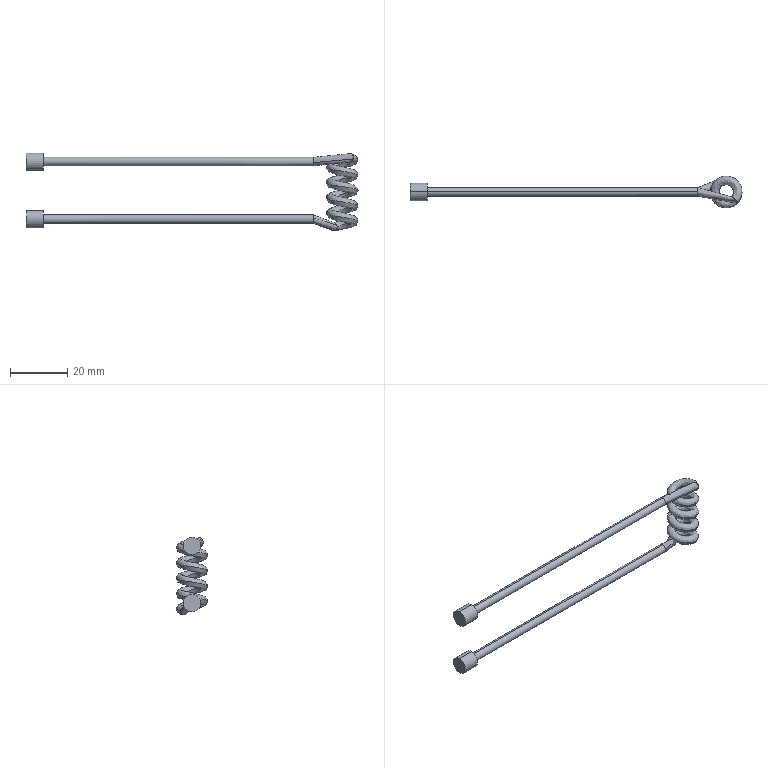Part | SolidWorks | features Blend 2, ICE 2, Fillet 1, Helix 1, Sweep 1 | 1 solid | 43 faces | box 115.5 x 11 x 27.126 mm | volume 2602 mm3 | spline 31 | cylinder 8 | plane 4 | commonest cylinder face diameters 3 x4 6 x4